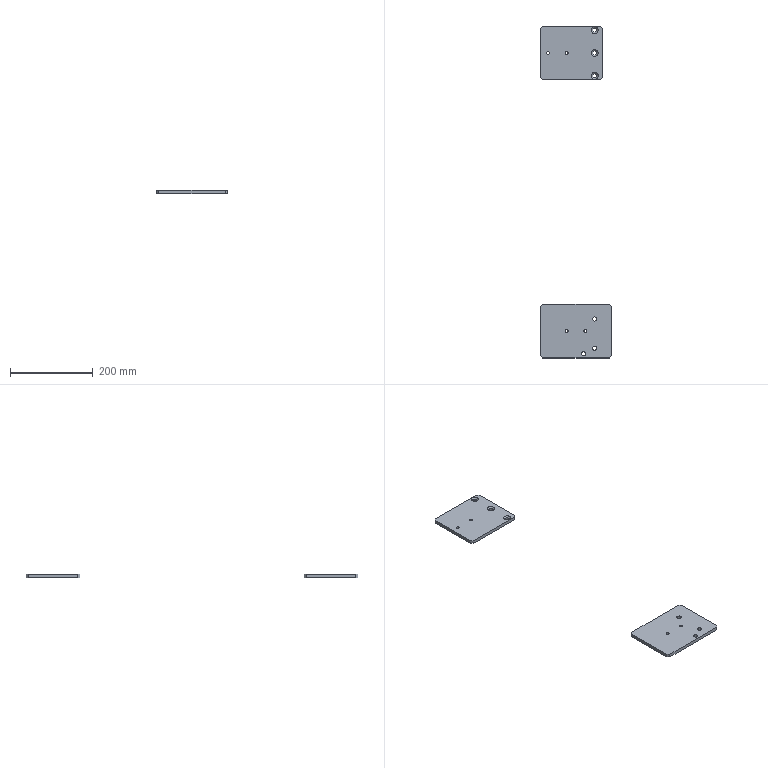Part | NX | features BREP 2 | 2 solids | 46 faces | box 170 x 800 x 8 mm | volume 326356 mm3 | cylinder 20 | plane 20 | cone 6 | commonest cylinder face diameters 10 x12 6.8 x8
STEP:
#1=CARTESIAN_POINT('',(23.429,-390.,0.));
#2=VERTEX_POINT('',#1);
#3=CARTESIAN_POINT('',(13.429,-390.,0.));
#4=VERTEX_POINT('',#3);
#5=CARTESIAN_POINT('',(18.429,-390.,0.));
#6=DIRECTION('',(0.,0.,-1.));
#7=DIRECTION('',(-1.,0.,0.));
#8=AXIS2_PLACEMENT_3D('',#5,#6,#7);
#9=CIRCLE('',#8,5.);
#10=EDGE_CURVE('',#2,#4,#9,.T.);
#11=ORIENTED_EDGE('',*,*,#10,.T.);
#12=CARTESIAN_POINT('',(13.429,-390.,8.));
#13=VERTEX_POINT('',#12);
#14=CARTESIAN_POINT('',(13.429,-390.,8.));
#15=DIRECTION('',(0.,0.,1.));
#16=VECTOR('',#15,1000.);
#17=LINE('',#14,#16);
#18=EDGE_CURVE('',#13,#4,#17,.F.);
#19=ORIENTED_EDGE('',*,*,#18,.F.);
#20=CARTESIAN_POINT('',(23.429,-390.,8.));
#21=VERTEX_POINT('',#20);
#22=CARTESIAN_POINT('',(18.429,-390.,8.));
#23=DIRECTION('',(0.,0.,1.));
#24=DIRECTION('',(1.,0.,0.));
#25=AXIS2_PLACEMENT_3D('',#22,#23,#24);
#26=CIRCLE('',#25,5.);
#27=EDGE_CURVE('',#13,#21,#26,.T.);
#28=ORIENTED_EDGE('',*,*,#27,.T.);
#29=CARTESIAN_POINT('',(23.429,-390.,8.));
#30=DIRECTION('',(0.,0.,1.));
#31=VECTOR('',#30,1000.);
#32=LINE('',#29,#31);
#33=EDGE_CURVE('',#21,#2,#32,.F.);
#34=ORIENTED_EDGE('',*,*,#33,.T.);
#35=EDGE_LOOP('',(#11,#19,#28,#34));
#36=FACE_BOUND('',#35,.T.);
#37=CARTESIAN_POINT('',(18.429,-390.,8.));
#38=DIRECTION('',(0.,0.,1.));
#39=DIRECTION('',(1.,0.,0.));
#40=AXIS2_PLACEMENT_3D('',#37,#38,#39);
#41=CYLINDRICAL_SURFACE('',#40,5.);
#42=ADVANCED_FACE('',(#36),#41,.F.);
#43=CARTESIAN_POINT('',(50.,-376.071,0.));
#44=VERTEX_POINT('',#43);
#45=CARTESIAN_POINT('',(40.,-376.071,0.));
#46=VERTEX_POINT('',#45);
#47=CARTESIAN_POINT('',(45.,-376.071,0.));
#48=DIRECTION('',(0.,0.,-1.));
#49=DIRECTION('',(-1.,0.,0.));
#50=AXIS2_PLACEMENT_3D('',#47,#48,#49);
#51=CIRCLE('',#50,5.);
#52=EDGE_CURVE('',#44,#46,#51,.T.);
#53=ORIENTED_EDGE('',*,*,#52,.T.);
#54=CARTESIAN_POINT('',(40.,-376.071,8.));
#55=VERTEX_POINT('',#54);
#56=CARTESIAN_POINT('',(40.,-376.071,8.));
#57=DIRECTION('',(0.,0.,1.));
#58=VECTOR('',#57,1000.);
#59=LINE('',#56,#58);
#60=EDGE_CURVE('',#55,#46,#59,.F.);
#61=ORIENTED_EDGE('',*,*,#60,.F.);
#62=CARTESIAN_POINT('',(50.,-376.071,8.));
#63=VERTEX_POINT('',#62);
#64=CARTESIAN_POINT('',(45.,-376.071,8.));
#65=DIRECTION('',(0.,0.,1.));
#66=DIRECTION('',(1.,0.,0.));
#67=AXIS2_PLACEMENT_3D('',#64,#65,#66);
#68=CIRCLE('',#67,5.);
#69=EDGE_CURVE('',#55,#63,#68,.T.);
#70=ORIENTED_EDGE('',*,*,#69,.T.);
#71=CARTESIAN_POINT('',(50.,-376.071,8.));
#72=DIRECTION('',(0.,0.,1.));
#73=VECTOR('',#72,1000.);
#74=LINE('',#71,#73);
#75=EDGE_CURVE('',#63,#44,#74,.F.);
#76=ORIENTED_EDGE('',*,*,#75,.T.);
#77=EDGE_LOOP('',(#53,#61,#70,#76));
#78=FACE_BOUND('',#77,.T.);
#79=CARTESIAN_POINT('',(45.,-376.071,8.));
#80=DIRECTION('',(0.,0.,1.));
#81=DIRECTION('',(1.,0.,0.));
#82=AXIS2_PLACEMENT_3D('',#79,#80,#81);
#83=CYLINDRICAL_SURFACE('',#82,5.);
#84=ADVANCED_FACE('',(#78),#83,.F.);
#85=CARTESIAN_POINT('',(50.,-306.071,0.));
#86=VERTEX_POINT('',#85);
#87=CARTESIAN_POINT('',(40.,-306.071,0.));
#88=VERTEX_POINT('',#87);
#89=CARTESIAN_POINT('',(45.,-306.071,0.));
#90=DIRECTION('',(0.,0.,-1.));
#91=DIRECTION('',(-1.,0.,0.));
#92=AXIS2_PLACEMENT_3D('',#89,#90,#91);
#93=CIRCLE('',#92,5.);
#94=EDGE_CURVE('',#86,#88,#93,.T.);
#95=ORIENTED_EDGE('',*,*,#94,.T.);
#96=CARTESIAN_POINT('',(40.,-306.071,8.));
#97=VERTEX_POINT('',#96);
#98=CARTESIAN_POINT('',(40.,-306.071,8.));
#99=DIRECTION('',(0.,0.,1.));
#100=VECTOR('',#99,1000.);
#101=LINE('',#98,#100);
#102=EDGE_CURVE('',#97,#88,#101,.F.);
#103=ORIENTED_EDGE('',*,*,#102,.F.);
#104=CARTESIAN_POINT('',(50.,-306.071,8.));
#105=VERTEX_POINT('',#104);
#106=CARTESIAN_POINT('',(45.,-306.071,8.));
#107=DIRECTION('',(0.,0.,1.));
#108=DIRECTION('',(1.,0.,0.));
#109=AXIS2_PLACEMENT_3D('',#106,#107,#108);
#110=CIRCLE('',#109,5.);
#111=EDGE_CURVE('',#97,#105,#110,.T.);
#112=ORIENTED_EDGE('',*,*,#111,.T.);
#113=CARTESIAN_POINT('',(50.,-306.071,8.));
#114=DIRECTION('',(0.,0.,1.));
#115=VECTOR('',#114,1000.);
#116=LINE('',#113,#115);
#117=EDGE_CURVE('',#105,#86,#116,.F.);
#118=ORIENTED_EDGE('',*,*,#117,.T.);
#119=EDGE_LOOP('',(#95,#103,#112,#118));
#120=FACE_BOUND('',#119,.T.);
#121=CARTESIAN_POINT('',(45.,-306.071,8.));
#122=DIRECTION('',(0.,0.,1.));
#123=DIRECTION('',(1.,0.,0.));
#124=AXIS2_PLACEMENT_3D('',#121,#122,#123);
#125=CYLINDRICAL_SURFACE('',#124,5.);
#126=ADVANCED_FACE('',(#120),#125,.F.);
#127=CARTESIAN_POINT('',(25.9,-335.,0.));
#128=VERTEX_POINT('',#127);
#129=CARTESIAN_POINT('',(19.1,-335.,0.));
#130=VERTEX_POINT('',#129);
#131=CARTESIAN_POINT('',(22.5,-335.,0.));
#132=DIRECTION('',(0.,0.,-1.));
#133=DIRECTION('',(-1.,0.,0.));
#134=AXIS2_PLACEMENT_3D('',#131,#132,#133);
#135=CIRCLE('',#134,3.4);
#136=EDGE_CURVE('',#128,#130,#135,.T.);
#137=ORIENTED_EDGE('',*,*,#136,.T.);
#138=CARTESIAN_POINT('',(19.1,-335.,8.));
#139=VERTEX_POINT('',#138);
#140=CARTESIAN_POINT('',(19.1,-335.,8.));
#141=DIRECTION('',(0.,0.,1.));
#142=VECTOR('',#141,1000.);
#143=LINE('',#140,#142);
#144=EDGE_CURVE('',#139,#130,#143,.F.);
#145=ORIENTED_EDGE('',*,*,#144,.F.);
#146=CARTESIAN_POINT('',(25.9,-335.,8.));
#147=VERTEX_POINT('',#146);
#148=CARTESIAN_POINT('',(22.5,-335.,8.));
#149=DIRECTION('',(0.,0.,1.));
#150=DIRECTION('',(1.,0.,0.));
#151=AXIS2_PLACEMENT_3D('',#148,#149,#150);
#152=CIRCLE('',#151,3.4);
#153=EDGE_CURVE('',#139,#147,#152,.T.);
#154=ORIENTED_EDGE('',*,*,#153,.T.);
#155=CARTESIAN_POINT('',(25.9,-335.,8.));
#156=DIRECTION('',(0.,0.,1.));
#157=VECTOR('',#156,1000.);
#158=LINE('',#155,#157);
#159=EDGE_CURVE('',#147,#128,#158,.F.);
#160=ORIENTED_EDGE('',*,*,#159,.T.);
#161=EDGE_LOOP('',(#137,#145,#154,#160));
#162=FACE_BOUND('',#161,.T.);
#163=CARTESIAN_POINT('',(22.5,-335.,8.));
#164=DIRECTION('',(0.,0.,1.));
#165=DIRECTION('',(1.,0.,0.));
#166=AXIS2_PLACEMENT_3D('',#163,#164,#165);
#167=CYLINDRICAL_SURFACE('',#166,3.4);
#168=ADVANCED_FACE('',(#162),#167,.F.);
#169=CARTESIAN_POINT('',(-19.1,-335.,0.));
#170=VERTEX_POINT('',#169);
#171=CARTESIAN_POINT('',(-25.9,-335.,0.));
#172=VERTEX_POINT('',#171);
#173=CARTESIAN_POINT('',(-22.5,-335.,0.));
#174=DIRECTION('',(0.,0.,-1.));
#175=DIRECTION('',(-1.,0.,0.));
#176=AXIS2_PLACEMENT_3D('',#173,#174,#175);
#177=CIRCLE('',#176,3.4);
#178=EDGE_CURVE('',#170,#172,#177,.T.);
#179=ORIENTED_EDGE('',*,*,#178,.T.);
#180=CARTESIAN_POINT('',(-25.9,-335.,8.));
#181=VERTEX_POINT('',#180);
#182=CARTESIAN_POINT('',(-25.9,-335.,8.));
#183=DIRECTION('',(0.,0.,1.));
#184=VECTOR('',#183,1000.);
#185=LINE('',#182,#184);
#186=EDGE_CURVE('',#181,#172,#185,.F.);
#187=ORIENTED_EDGE('',*,*,#186,.F.);
#188=CARTESIAN_POINT('',(-19.1,-335.,8.));
#189=VERTEX_POINT('',#188);
#190=CARTESIAN_POINT('',(-22.5,-335.,8.));
#191=DIRECTION('',(0.,0.,1.));
#192=DIRECTION('',(1.,0.,0.));
#193=AXIS2_PLACEMENT_3D('',#190,#191,#192);
#194=CIRCLE('',#193,3.4);
#195=EDGE_CURVE('',#181,#189,#194,.T.);
#196=ORIENTED_EDGE('',*,*,#195,.T.);
#197=CARTESIAN_POINT('',(-19.1,-335.,8.));
#198=DIRECTION('',(0.,0.,1.));
#199=VECTOR('',#198,1000.);
#200=LINE('',#197,#199);
#201=EDGE_CURVE('',#189,#170,#200,.F.);
#202=ORIENTED_EDGE('',*,*,#201,.T.);
#203=EDGE_LOOP('',(#179,#187,#196,#202));
#204=FACE_BOUND('',#203,.T.);
#205=CARTESIAN_POINT('',(-22.5,-335.,8.));
#206=DIRECTION('',(0.,0.,1.));
#207=DIRECTION('',(1.,0.,0.));
#208=AXIS2_PLACEMENT_3D('',#205,#206,#207);
#209=CYLINDRICAL_SURFACE('',#208,3.4);
#210=ADVANCED_FACE('',(#204),#209,.F.);
#211=CARTESIAN_POINT('',(85.,-395.,8.));
#212=VERTEX_POINT('',#211);
#213=CARTESIAN_POINT('',(85.,-275.,8.));
#214=VERTEX_POINT('',#213);
#215=CARTESIAN_POINT('',(85.,-400.,8.));
#216=DIRECTION('',(0.,1.,0.));
#217=VECTOR('',#216,1000.);
#218=LINE('',#215,#217);
#219=EDGE_CURVE('',#212,#214,#218,.T.);
#220=ORIENTED_EDGE('',*,*,#219,.F.);
#221=CARTESIAN_POINT('',(85.,-395.,0.));
#222=VERTEX_POINT('',#221);
#223=CARTESIAN_POINT('',(85.,-395.,8.));
#224=DIRECTION('',(0.,0.,-1.));
#225=VECTOR('',#224,1000.);
#226=LINE('',#223,#225);
#227=EDGE_CURVE('',#212,#222,#226,.T.);
#228=ORIENTED_EDGE('',*,*,#227,.T.);
#229=CARTESIAN_POINT('',(85.,-275.,0.));
#230=VERTEX_POINT('',#229);
#231=CARTESIAN_POINT('',(85.,-400.,0.));
#232=DIRECTION('',(0.,1.,0.));
#233=VECTOR('',#232,1000.);
#234=LINE('',#231,#233);
#235=EDGE_CURVE('',#222,#230,#234,.T.);
#236=ORIENTED_EDGE('',*,*,#235,.T.);
#237=CARTESIAN_POINT('',(85.,-275.,8.));
#238=DIRECTION('',(0.,0.,1.));
#239=VECTOR('',#238,1000.);
#240=LINE('',#237,#239);
#241=EDGE_CURVE('',#230,#214,#240,.T.);
#242=ORIENTED_EDGE('',*,*,#241,.T.);
#243=EDGE_LOOP('',(#220,#228,#236,#242));
#244=FACE_BOUND('',#243,.T.);
#245=CARTESIAN_POINT('',(85.,-400.,8.));
#246=DIRECTION('',(-1.,0.,0.));
#247=DIRECTION('',(0.,0.,1.));
#248=AXIS2_PLACEMENT_3D('',#245,#246,#247);
#249=PLANE('',#248);
#250=ADVANCED_FACE('',(#244),#249,.F.);
#251=CARTESIAN_POINT('',(-85.,-275.,0.));
#252=VERTEX_POINT('',#251);
#253=CARTESIAN_POINT('',(-85.,-395.,0.));
#254=VERTEX_POINT('',#253);
#255=CARTESIAN_POINT('',(-85.,-400.,0.));
#256=DIRECTION('',(0.,-1.,0.));
#257=VECTOR('',#256,1000.);
#258=LINE('',#255,#257);
#259=EDGE_CURVE('',#252,#254,#258,.T.);
#260=ORIENTED_EDGE('',*,*,#259,.T.);
#261=CARTESIAN_POINT('',(-85.,-395.,8.));
#262=VERTEX_POINT('',#261);
#263=CARTESIAN_POINT('',(-85.,-395.,8.));
#264=DIRECTION('',(0.,0.,1.));
#265=VECTOR('',#264,1000.);
#266=LINE('',#263,#265);
#267=EDGE_CURVE('',#254,#262,#266,.T.);
#268=ORIENTED_EDGE('',*,*,#267,.T.);
#269=CARTESIAN_POINT('',(-85.,-275.,8.));
#270=VERTEX_POINT('',#269);
#271=CARTESIAN_POINT('',(-85.,-400.,8.));
#272=DIRECTION('',(0.,-1.,0.));
#273=VECTOR('',#272,1000.);
#274=LINE('',#271,#273);
#275=EDGE_CURVE('',#270,#262,#274,.T.);
#276=ORIENTED_EDGE('',*,*,#275,.F.);
#277=CARTESIAN_POINT('',(-85.,-275.,8.));
#278=DIRECTION('',(0.,0.,-1.));
#279=VECTOR('',#278,1000.);
#280=LINE('',#277,#279);
#281=EDGE_CURVE('',#270,#252,#280,.T.);
#282=ORIENTED_EDGE('',*,*,#281,.T.);
#283=EDGE_LOOP('',(#260,#268,#276,#282));
#284=FACE_BOUND('',#283,.T.);
#285=CARTESIAN_POINT('',(-85.,-400.,8.));
#286=DIRECTION('',(1.,0.,0.));
#287=DIRECTION('',(0.,1.,0.));
#288=AXIS2_PLACEMENT_3D('',#285,#286,#287);
#289=PLANE('',#288);
#290=ADVANCED_FACE('',(#284),#289,.F.);
#291=CARTESIAN_POINT('',(-80.,-400.,8.));
#292=VERTEX_POINT('',#291);
#293=CARTESIAN_POINT('',(80.,-400.,8.));
#294=VERTEX_POINT('',#293);
#295=CARTESIAN_POINT('',(-85.,-400.,8.));
#296=DIRECTION('',(1.,0.,0.));
#297=VECTOR('',#296,1000.);
#298=LINE('',#295,#297);
#299=EDGE_CURVE('',#292,#294,#298,.T.);
#300=ORIENTED_EDGE('',*,*,#299,.T.);
#301=CARTESIAN_POINT('',(85.,-395.,8.));
#302=DIRECTION('',(0.7071,0.7071,0.));
#303=VECTOR('',#302,1000.);
#304=LINE('',#301,#303);
#305=EDGE_CURVE('',#294,#212,#304,.T.);
#306=ORIENTED_EDGE('',*,*,#305,.T.);
#307=ORIENTED_EDGE('',*,*,#219,.T.);
#308=CARTESIAN_POINT('',(80.,-270.,8.));
#309=VERTEX_POINT('',#308);
#310=CARTESIAN_POINT('',(85.,-275.,8.));
#311=DIRECTION('',(-0.7071,0.7071,0.));
#312=VECTOR('',#311,1000.);
#313=LINE('',#310,#312);
#314=EDGE_CURVE('',#214,#309,#313,.T.);
#315=ORIENTED_EDGE('',*,*,#314,.T.);
#316=CARTESIAN_POINT('',(-80.,-270.,8.));
#317=VERTEX_POINT('',#316);
#318=CARTESIAN_POINT('',(-85.,-270.,8.));
#319=DIRECTION('',(1.,0.,0.));
#320=VECTOR('',#319,1000.);
#321=LINE('',#318,#320);
#322=EDGE_CURVE('',#317,#309,#321,.T.);
#323=ORIENTED_EDGE('',*,*,#322,.F.);
#324=CARTESIAN_POINT('',(-80.,-270.,8.));
#325=DIRECTION('',(-0.7071,-0.7071,0.));
#326=VECTOR('',#325,1000.);
#327=LINE('',#324,#326);
#328=EDGE_CURVE('',#317,#270,#327,.T.);
#329=ORIENTED_EDGE('',*,*,#328,.T.);
#330=ORIENTED_EDGE('',*,*,#275,.T.);
#331=CARTESIAN_POINT('',(-80.,-400.,8.));
#332=DIRECTION('',(0.7071,-0.7071,0.));
#333=VECTOR('',#332,1000.);
#334=LINE('',#331,#333);
#335=EDGE_CURVE('',#262,#292,#334,.T.);
#336=ORIENTED_EDGE('',*,*,#335,.T.);
#337=EDGE_LOOP('',(#300,#306,#307,#315,#323,#329,#330,#336));
#338=FACE_BOUND('',#337,.T.);
#339=CARTESIAN_POINT('',(-22.5,-335.,8.));
#340=DIRECTION('',(0.,0.,1.));
#341=DIRECTION('',(1.,0.,0.));
#342=AXIS2_PLACEMENT_3D('',#339,#340,#341);
#343=CIRCLE('',#342,3.4);
#344=EDGE_CURVE('',#189,#181,#343,.T.);
#345=ORIENTED_EDGE('',*,*,#344,.F.);
#346=ORIENTED_EDGE('',*,*,#195,.F.);
#347=EDGE_LOOP('',(#345,#346));
#348=FACE_BOUND('',#347,.T.);
#349=CARTESIAN_POINT('',(22.5,-335.,8.));
#350=DIRECTION('',(0.,0.,1.));
#351=DIRECTION('',(1.,0.,0.));
#352=AXIS2_PLACEMENT_3D('',#349,#350,#351);
#353=CIRCLE('',#352,3.4);
#354=EDGE_CURVE('',#147,#139,#353,.T.);
#355=ORIENTED_EDGE('',*,*,#354,.F.);
#356=ORIENTED_EDGE('',*,*,#153,.F.);
#357=EDGE_LOOP('',(#355,#356));
#358=FACE_BOUND('',#357,.T.);
#359=CARTESIAN_POINT('',(45.,-306.071,8.));
#360=DIRECTION('',(0.,0.,1.));
#361=DIRECTION('',(1.,0.,0.));
#362=AXIS2_PLACEMENT_3D('',#359,#360,#361);
#363=CIRCLE('',#362,5.);
#364=EDGE_CURVE('',#105,#97,#363,.T.);
#365=ORIENTED_EDGE('',*,*,#364,.F.);
#366=ORIENTED_EDGE('',*,*,#111,.F.);
#367=EDGE_LOOP('',(#365,#366));
#368=FACE_BOUND('',#367,.T.);
#369=CARTESIAN_POINT('',(45.,-376.071,8.));
#370=DIRECTION('',(0.,0.,1.));
#371=DIRECTION('',(1.,0.,0.));
#372=AXIS2_PLACEMENT_3D('',#369,#370,#371);
#373=CIRCLE('',#372,5.);
#374=EDGE_CURVE('',#63,#55,#373,.T.);
#375=ORIENTED_EDGE('',*,*,#374,.F.);
#376=ORIENTED_EDGE('',*,*,#69,.F.);
#377=EDGE_LOOP('',(#375,#376));
#378=FACE_BOUND('',#377,.T.);
#379=CARTESIAN_POINT('',(18.429,-390.,8.));
#380=DIRECTION('',(0.,0.,1.));
#381=DIRECTION('',(1.,0.,0.));
#382=AXIS2_PLACEMENT_3D('',#379,#380,#381);
#383=CIRCLE('',#382,5.);
#384=EDGE_CURVE('',#21,#13,#383,.T.);
#385=ORIENTED_EDGE('',*,*,#384,.F.);
#386=ORIENTED_EDGE('',*,*,#27,.F.);
#387=EDGE_LOOP('',(#385,#386));
#388=FACE_BOUND('',#387,.T.);
#389=CARTESIAN_POINT('',(0.,0.,8.));
#390=DIRECTION('',(0.,0.,-1.));
#391=DIRECTION('',(0.,-1.,0.));
#392=AXIS2_PLACEMENT_3D('',#389,#390,#391);
#393=PLANE('',#392);
#394=ADVANCED_FACE('',(#338,#348,#358,#368,#378,#388),#393,.F.);
#395=ORIENTED_EDGE('',*,*,#235,.F.);
#396=CARTESIAN_POINT('',(80.,-400.,0.));
#397=VERTEX_POINT('',#396);
#398=CARTESIAN_POINT('',(240.,-240.,0.));
#399=DIRECTION('',(-0.7071,-0.7071,0.));
#400=VECTOR('',#399,1000.);
#401=LINE('',#398,#400);
#402=EDGE_CURVE('',#222,#397,#401,.T.);
#403=ORIENTED_EDGE('',*,*,#402,.T.);
#404=CARTESIAN_POINT('',(-80.,-400.,0.));
#405=VERTEX_POINT('',#404);
#406=CARTESIAN_POINT('',(-85.,-400.,0.));
#407=DIRECTION('',(1.,0.,0.));
#408=VECTOR('',#407,1000.);
#409=LINE('',#406,#408);
#410=EDGE_CURVE('',#405,#397,#409,.T.);
#411=ORIENTED_EDGE('',*,*,#410,.F.);
#412=CARTESIAN_POINT('',(-240.,-240.,0.));
#413=DIRECTION('',(-0.7071,0.7071,0.));
#414=VECTOR('',#413,1000.);
#415=LINE('',#412,#414);
#416=EDGE_CURVE('',#405,#254,#415,.T.);
#417=ORIENTED_EDGE('',*,*,#416,.T.);
#418=ORIENTED_EDGE('',*,*,#259,.F.);
#419=CARTESIAN_POINT('',(-80.,-270.,0.));
#420=VERTEX_POINT('',#419);
#421=CARTESIAN_POINT('',(95.,-95.,0.));
#422=DIRECTION('',(0.7071,0.7071,0.));
#423=VECTOR('',#422,1000.);
#424=LINE('',#421,#423);
#425=EDGE_CURVE('',#252,#420,#424,.T.);
#426=ORIENTED_EDGE('',*,*,#425,.T.);
#427=CARTESIAN_POINT('',(80.,-270.,0.));
#428=VERTEX_POINT('',#427);
#429=CARTESIAN_POINT('',(0.,-270.,0.));
#430=DIRECTION('',(-1.,0.,0.));
#431=VECTOR('',#430,1000.);
#432=LINE('',#429,#431);
#433=EDGE_CURVE('',#428,#420,#432,.T.);
#434=ORIENTED_EDGE('',*,*,#433,.F.);
#435=CARTESIAN_POINT('',(-95.,-95.,0.));
#436=DIRECTION('',(0.7071,-0.7071,0.));
#437=VECTOR('',#436,1000.);
#438=LINE('',#435,#437);
#439=EDGE_CURVE('',#428,#230,#438,.T.);
#440=ORIENTED_EDGE('',*,*,#439,.T.);
#441=EDGE_LOOP('',(#395,#403,#411,#417,#418,#426,#434,#440));
#442=FACE_BOUND('',#441,.T.);
#443=ORIENTED_EDGE('',*,*,#178,.F.);
#444=CARTESIAN_POINT('',(-22.5,-335.,0.));
#445=DIRECTION('',(0.,0.,-1.));
#446=DIRECTION('',(-1.,0.,0.));
#447=AXIS2_PLACEMENT_3D('',#444,#445,#446);
#448=CIRCLE('',#447,3.4);
#449=EDGE_CURVE('',#172,#170,#448,.T.);
#450=ORIENTED_EDGE('',*,*,#449,.F.);
#451=EDGE_LOOP('',(#443,#450));
#452=FACE_BOUND('',#451,.T.);
#453=ORIENTED_EDGE('',*,*,#136,.F.);
#454=CARTESIAN_POINT('',(22.5,-335.,0.));
#455=DIRECTION('',(0.,0.,-1.));
#456=DIRECTION('',(-1.,0.,0.));
#457=AXIS2_PLACEMENT_3D('',#454,#455,#456);
#458=CIRCLE('',#457,3.4);
#459=EDGE_CURVE('',#130,#128,#458,.T.);
#460=ORIENTED_EDGE('',*,*,#459,.F.);
#461=EDGE_LOOP('',(#453,#460));
#462=FACE_BOUND('',#461,.T.);
#463=ORIENTED_EDGE('',*,*,#94,.F.);
#464=CARTESIAN_POINT('',(45.,-306.071,0.));
#465=DIRECTION('',(0.,0.,-1.));
#466=DIRECTION('',(-1.,0.,0.));
#467=AXIS2_PLACEMENT_3D('',#464,#465,#466);
#468=CIRCLE('',#467,5.);
#469=EDGE_CURVE('',#88,#86,#468,.T.);
#470=ORIENTED_EDGE('',*,*,#469,.F.);
#471=EDGE_LOOP('',(#463,#470));
#472=FACE_BOUND('',#471,.T.);
#473=ORIENTED_EDGE('',*,*,#52,.F.);
#474=CARTESIAN_POINT('',(45.,-376.071,0.));
#475=DIRECTION('',(0.,0.,-1.));
#476=DIRECTION('',(-1.,0.,0.));
#477=AXIS2_PLACEMENT_3D('',#474,#475,#476);
#478=CIRCLE('',#477,5.);
#479=EDGE_CURVE('',#46,#44,#478,.T.);
#480=ORIENTED_EDGE('',*,*,#479,.F.);
#481=EDGE_LOOP('',(#473,#480));
#482=FACE_BOUND('',#481,.T.);
#483=ORIENTED_EDGE('',*,*,#10,.F.);
#484=CARTESIAN_POINT('',(18.429,-390.,0.));
#485=DIRECTION('',(0.,0.,-1.));
#486=DIRECTION('',(-1.,0.,0.));
#487=AXIS2_PLACEMENT_3D('',#484,#485,#486);
#488=CIRCLE('',#487,5.);
#489=EDGE_CURVE('',#4,#2,#488,.T.);
#490=ORIENTED_EDGE('',*,*,#489,.F.);
#491=EDGE_LOOP('',(#483,#490));
#492=FACE_BOUND('',#491,.T.);
#493=CARTESIAN_POINT('',(0.,0.,0.));
#494=DIRECTION('',(0.,0.,-1.));
#495=DIRECTION('',(0.,-1.,0.));
#496=AXIS2_PLACEMENT_3D('',#493,#494,#495);
#497=PLANE('',#496);
#498=ADVANCED_FACE('',(#442,#452,#462,#472,#482,#492),#497,.T.);
#499=ORIENTED_EDGE('',*,*,#410,.T.);
#500=CARTESIAN_POINT('',(80.,-400.,8.));
#501=DIRECTION('',(0.,0.,1.));
#502=VECTOR('',#501,1000.);
#503=LINE('',#500,#502);
#504=EDGE_CURVE('',#397,#294,#503,.T.);
#505=ORIENTED_EDGE('',*,*,#504,.T.);
#506=ORIENTED_EDGE('',*,*,#299,.F.);
#507=CARTESIAN_POINT('',(-80.,-400.,8.));
#508=DIRECTION('',(0.,0.,-1.));
#509=VECTOR('',#508,1000.);
#510=LINE('',#507,#509);
#511=EDGE_CURVE('',#292,#405,#510,.T.);
#512=ORIENTED_EDGE('',*,*,#511,.T.);
#513=EDGE_LOOP('',(#499,#505,#506,#512));
#514=FACE_BOUND('',#513,.T.);
#515=CARTESIAN_POINT('',(-85.,-400.,8.));
#516=DIRECTION('',(0.,1.,0.));
#517=DIRECTION('',(1.,0.,0.));
#518=AXIS2_PLACEMENT_3D('',#515,#516,#517);
#519=PLANE('',#518);
#520=ADVANCED_FACE('',(#514),#519,.F.);
#521=ORIENTED_EDGE('',*,*,#186,.T.);
#522=ORIENTED_EDGE('',*,*,#449,.T.);
#523=ORIENTED_EDGE('',*,*,#201,.F.);
#524=ORIENTED_EDGE('',*,*,#344,.T.);
#525=EDGE_LOOP('',(#521,#522,#523,#524));
#526=FACE_BOUND('',#525,.T.);
#527=CARTESIAN_POINT('',(-22.5,-335.,8.));
#528=DIRECTION('',(0.,0.,1.));
#529=DIRECTION('',(1.,0.,0.));
#530=AXIS2_PLACEMENT_3D('',#527,#528,#529);
#531=CYLINDRICAL_SURFACE('',#530,3.4);
#532=ADVANCED_FACE('',(#526),#531,.F.);
#533=ORIENTED_EDGE('',*,*,#144,.T.);
#534=ORIENTED_EDGE('',*,*,#459,.T.);
#535=ORIENTED_EDGE('',*,*,#159,.F.);
#536=ORIENTED_EDGE('',*,*,#354,.T.);
#537=EDGE_LOOP('',(#533,#534,#535,#536));
#538=FACE_BOUND('',#537,.T.);
#539=CARTESIAN_POINT('',(22.5,-335.,8.));
#540=DIRECTION('',(0.,0.,1.));
#541=DIRECTION('',(1.,0.,0.));
#542=AXIS2_PLACEMENT_3D('',#539,#540,#541);
#543=CYLINDRICAL_SURFACE('',#542,3.4);
#544=ADVANCED_FACE('',(#538),#543,.F.);
#545=ORIENTED_EDGE('',*,*,#102,.T.);
#546=ORIENTED_EDGE('',*,*,#469,.T.);
#547=ORIENTED_EDGE('',*,*,#117,.F.);
#548=ORIENTED_EDGE('',*,*,#364,.T.);
#549=EDGE_LOOP('',(#545,#546,#547,#548));
#550=FACE_BOUND('',#549,.T.);
#551=CARTESIAN_POINT('',(45.,-306.071,8.));
#552=DIRECTION('',(0.,0.,1.));
#553=DIRECTION('',(1.,0.,0.));
#554=AXIS2_PLACEMENT_3D('',#551,#552,#553);
#555=CYLINDRICAL_SURFACE('',#554,5.);
#556=ADVANCED_FACE('',(#550),#555,.F.);
#557=ORIENTED_EDGE('',*,*,#60,.T.);
#558=ORIENTED_EDGE('',*,*,#479,.T.);
#559=ORIENTED_EDGE('',*,*,#75,.F.);
#560=ORIENTED_EDGE('',*,*,#374,.T.);
#561=EDGE_LOOP('',(#557,#558,#559,#560));
#562=FACE_BOUND('',#561,.T.);
#563=CARTESIAN_POINT('',(45.,-376.071,8.));
#564=DIRECTION('',(0.,0.,1.));
#565=DIRECTION('',(1.,0.,0.));
#566=AXIS2_PLACEMENT_3D('',#563,#564,#565);
#567=CYLINDRICAL_SURFACE('',#566,5.);
#568=ADVANCED_FACE('',(#562),#567,.F.);
#569=ORIENTED_EDGE('',*,*,#18,.T.);
#570=ORIENTED_EDGE('',*,*,#489,.T.);
#571=ORIENTED_EDGE('',*,*,#33,.F.);
#572=ORIENTED_EDGE('',*,*,#384,.T.);
#573=EDGE_LOOP('',(#569,#570,#571,#572));
#574=FACE_BOUND('',#573,.T.);
#575=CARTESIAN_POINT('',(18.429,-390.,8.));
#576=DIRECTION('',(0.,0.,1.));
#577=DIRECTION('',(1.,0.,0.));
#578=AXIS2_PLACEMENT_3D('',#575,#576,#577);
#579=CYLINDRICAL_SURFACE('',#578,5.);
#580=ADVANCED_FACE('',(#574),#579,.F.);
#581=ORIENTED_EDGE('',*,*,#433,.T.);
#582=CARTESIAN_POINT('',(-80.,-270.,-2.));
#583=DIRECTION('',(0.,0.,1.));
#584=VECTOR('',#583,1000.);
#585=LINE('',#582,#584);
#586=EDGE_CURVE('',#420,#317,#585,.T.);
#587=ORIENTED_EDGE('',*,*,#586,.T.);
#588=ORIENTED_EDGE('',*,*,#322,.T.);
#589=CARTESIAN_POINT('',(80.,-270.,-2.));
#590=DIRECTION('',(0.,0.,-1.));
#591=VECTOR('',#590,1000.);
#592=LINE('',#589,#591);
#593=EDGE_CURVE('',#309,#428,#592,.T.);
#594=ORIENTED_EDGE('',*,*,#593,.T.);
#595=EDGE_LOOP('',(#581,#587,#588,#594));
#596=FACE_BOUND('',#595,.T.);
#597=CARTESIAN_POINT('',(-85.,-270.,-2.));
#598=DIRECTION('',(0.,-1.,0.));
#599=DIRECTION('',(0.,0.,-1.));
#600=AXIS2_PLACEMENT_3D('',#597,#598,#599);
#601=PLANE('',#600);
#602=ADVANCED_FACE('',(#596),#601,.F.);
#603=ORIENTED_EDGE('',*,*,#305,.F.);
#604=ORIENTED_EDGE('',*,*,#504,.F.);
#605=ORIENTED_EDGE('',*,*,#402,.F.);
#606=ORIENTED_EDGE('',*,*,#227,.F.);
#607=EDGE_LOOP('',(#603,#604,#605,#606));
#608=FACE_BOUND('',#607,.T.);
#609=CARTESIAN_POINT('',(85.,-395.,8.));
#610=DIRECTION('',(-0.7071,0.7071,0.));
#611=DIRECTION('',(0.,0.,1.));
#612=AXIS2_PLACEMENT_3D('',#609,#610,#611);
#613=PLANE('',#612);
#614=ADVANCED_FACE('',(#608),#613,.F.);
#615=ORIENTED_EDGE('',*,*,#335,.F.);
#616=ORIENTED_EDGE('',*,*,#267,.F.);
#617=ORIENTED_EDGE('',*,*,#416,.F.);
#618=ORIENTED_EDGE('',*,*,#511,.F.);
#619=EDGE_LOOP('',(#615,#616,#617,#618));
#620=FACE_BOUND('',#619,.T.);
#621=CARTESIAN_POINT('',(-80.,-400.,8.));
#622=DIRECTION('',(0.7071,0.7071,0.));
#623=DIRECTION('',(0.,0.,-1.));
#624=AXIS2_PLACEMENT_3D('',#621,#622,#623);
#625=PLANE('',#624);
#626=ADVANCED_FACE('',(#620),#625,.F.);
#627=ORIENTED_EDGE('',*,*,#425,.F.);
#628=ORIENTED_EDGE('',*,*,#281,.F.);
#629=ORIENTED_EDGE('',*,*,#328,.F.);
#630=ORIENTED_EDGE('',*,*,#586,.F.);
#631=EDGE_LOOP('',(#627,#628,#629,#630));
#632=FACE_BOUND('',#631,.T.);
#633=CARTESIAN_POINT('',(-80.,-270.,-2.));
#634=DIRECTION('',(0.7071,-0.7071,0.));
#635=DIRECTION('',(0.,0.,-1.));
#636=AXIS2_PLACEMENT_3D('',#633,#634,#635);
#637=PLANE('',#636);
#638=ADVANCED_FACE('',(#632),#637,.F.);
#639=ORIENTED_EDGE('',*,*,#439,.F.);
#640=ORIENTED_EDGE('',*,*,#593,.F.);
#641=ORIENTED_EDGE('',*,*,#314,.F.);
#642=ORIENTED_EDGE('',*,*,#241,.F.);
#643=EDGE_LOOP('',(#639,#640,#641,#642));
#644=FACE_BOUND('',#643,.T.);
#645=CARTESIAN_POINT('',(85.,-275.,8.));
#646=DIRECTION('',(-0.7071,-0.7071,0.));
#647=DIRECTION('',(-0.7071,0.7071,0.));
#648=AXIS2_PLACEMENT_3D('',#645,#646,#647);
#649=PLANE('',#648);
#650=ADVANCED_FACE('',(#644),#649,.F.);
#651=CLOSED_SHELL('',(#42,#84,#126,#168,#210,#250,#290,#394,#498,#520,#532,#544,#556,#568,#580,#602,#614,#626,#638,#650));
#652=MANIFOLD_SOLID_BREP('',#651);
#653=CARTESIAN_POINT('',(40.,390.,4.5));
#654=VERTEX_POINT('',#653);
#655=CARTESIAN_POINT('',(50.,390.,4.5));
#656=VERTEX_POINT('',#655);
#657=CARTESIAN_POINT('',(45.,390.,4.5));
#658=DIRECTION('',(0.,0.,1.));
#659=DIRECTION('',(-1.,0.,0.));
#660=AXIS2_PLACEMENT_3D('',#657,#658,#659);
#661=CIRCLE('',#660,5.);
#662=EDGE_CURVE('',#654,#656,#661,.T.);
#663=ORIENTED_EDGE('',*,*,#662,.F.);
#664=CARTESIAN_POINT('',(36.5,390.,8.));
#665=VERTEX_POINT('',#664);
#666=CARTESIAN_POINT('',(40.,390.,4.5));
#667=DIRECTION('',(-0.7071,0.,0.7071));
#668=VECTOR('',#667,1000.);
#669=LINE('',#666,#668);
#670=EDGE_CURVE('',#665,#654,#669,.F.);
#671=ORIENTED_EDGE('',*,*,#670,.F.);
#672=CARTESIAN_POINT('',(53.5,390.,8.));
#673=VERTEX_POINT('',#672);
#674=CARTESIAN_POINT('',(45.,390.,8.));
#675=DIRECTION('',(0.,0.,-1.));
#676=DIRECTION('',(-1.,0.,0.));
#677=AXIS2_PLACEMENT_3D('',#674,#675,#676);
#678=CIRCLE('',#677,8.5);
#679=EDGE_CURVE('',#673,#665,#678,.T.);
#680=ORIENTED_EDGE('',*,*,#679,.F.);
#681=CARTESIAN_POINT('',(50.,390.,4.5));
#682=DIRECTION('',(0.7071,0.,0.7071));
#683=VECTOR('',#682,1000.);
#684=LINE('',#681,#683);
#685=EDGE_CURVE('',#673,#656,#684,.F.);
#686=ORIENTED_EDGE('',*,*,#685,.T.);
#687=EDGE_LOOP('',(#663,#671,#680,#686));
#688=FACE_BOUND('',#687,.T.);
#689=CARTESIAN_POINT('',(45.,390.,4.5));
#690=DIRECTION('',(0.,0.,1.));
#691=DIRECTION('',(1.,0.,0.));
#692=AXIS2_PLACEMENT_3D('',#689,#690,#691);
#693=CONICAL_SURFACE('',#692,5.,0.7854);
#694=ADVANCED_FACE('',(#688),#693,.F.);
#695=CARTESIAN_POINT('',(40.,335.,4.5));
#696=VERTEX_POINT('',#695);
#697=CARTESIAN_POINT('',(50.,335.,4.5));
#698=VERTEX_POINT('',#697);
#699=CARTESIAN_POINT('',(45.,335.,4.5));
#700=DIRECTION('',(0.,0.,1.));
#701=DIRECTION('',(-1.,0.,0.));
#702=AXIS2_PLACEMENT_3D('',#699,#700,#701);
#703=CIRCLE('',#702,5.);
#704=EDGE_CURVE('',#696,#698,#703,.T.);
#705=ORIENTED_EDGE('',*,*,#704,.F.);
#706=CARTESIAN_POINT('',(36.5,335.,8.));
#707=VERTEX_POINT('',#706);
#708=CARTESIAN_POINT('',(40.,335.,4.5));
#709=DIRECTION('',(-0.7071,0.,0.7071));
#710=VECTOR('',#709,1000.);
#711=LINE('',#708,#710);
#712=EDGE_CURVE('',#707,#696,#711,.F.);
#713=ORIENTED_EDGE('',*,*,#712,.F.);
#714=CARTESIAN_POINT('',(53.5,335.,8.));
#715=VERTEX_POINT('',#714);
#716=CARTESIAN_POINT('',(45.,335.,8.));
#717=DIRECTION('',(0.,0.,-1.));
#718=DIRECTION('',(-1.,0.,0.));
#719=AXIS2_PLACEMENT_3D('',#716,#717,#718);
#720=CIRCLE('',#719,8.5);
#721=EDGE_CURVE('',#715,#707,#720,.T.);
#722=ORIENTED_EDGE('',*,*,#721,.F.);
#723=CARTESIAN_POINT('',(50.,335.,4.5));
#724=DIRECTION('',(0.7071,0.,0.7071));
#725=VECTOR('',#724,1000.);
#726=LINE('',#723,#725);
#727=EDGE_CURVE('',#715,#698,#726,.F.);
#728=ORIENTED_EDGE('',*,*,#727,.T.);
#729=EDGE_LOOP('',(#705,#713,#722,#728));
#730=FACE_BOUND('',#729,.T.);
#731=CARTESIAN_POINT('',(45.,335.,4.5));
#732=DIRECTION('',(0.,0.,1.));
#733=DIRECTION('',(1.,0.,0.));
#734=AXIS2_PLACEMENT_3D('',#731,#732,#733);
#735=CONICAL_SURFACE('',#734,5.,0.7854);
#736=ADVANCED_FACE('',(#730),#735,.F.);
#737=CARTESIAN_POINT('',(40.,280.,4.5));
#738=VERTEX_POINT('',#737);
#739=CARTESIAN_POINT('',(50.,280.,4.5));
#740=VERTEX_POINT('',#739);
#741=CARTESIAN_POINT('',(45.,280.,4.5));
#742=DIRECTION('',(0.,0.,1.));
#743=DIRECTION('',(-1.,0.,0.));
#744=AXIS2_PLACEMENT_3D('',#741,#742,#743);
#745=CIRCLE('',#744,5.);
#746=EDGE_CURVE('',#738,#740,#745,.T.);
#747=ORIENTED_EDGE('',*,*,#746,.F.);
#748=CARTESIAN_POINT('',(36.5,280.,8.));
#749=VERTEX_POINT('',#748);
#750=CARTESIAN_POINT('',(40.,280.,4.5));
#751=DIRECTION('',(-0.7071,0.,0.7071));
#752=VECTOR('',#751,1000.);
#753=LINE('',#750,#752);
#754=EDGE_CURVE('',#749,#738,#753,.F.);
#755=ORIENTED_EDGE('',*,*,#754,.F.);
#756=CARTESIAN_POINT('',(53.5,280.,8.));
#757=VERTEX_POINT('',#756);
#758=CARTESIAN_POINT('',(45.,280.,8.));
#759=DIRECTION('',(0.,0.,-1.));
#760=DIRECTION('',(-1.,0.,0.));
#761=AXIS2_PLACEMENT_3D('',#758,#759,#760);
#762=CIRCLE('',#761,8.5);
#763=EDGE_CURVE('',#757,#749,#762,.T.);
#764=ORIENTED_EDGE('',*,*,#763,.F.);
#765=CARTESIAN_POINT('',(50.,280.,4.5));
#766=DIRECTION('',(0.7071,0.,0.7071));
#767=VECTOR('',#766,1000.);
#768=LINE('',#765,#767);
#769=EDGE_CURVE('',#757,#740,#768,.F.);
#770=ORIENTED_EDGE('',*,*,#769,.T.);
#771=EDGE_LOOP('',(#747,#755,#764,#770));
#772=FACE_BOUND('',#771,.T.);
#773=CARTESIAN_POINT('',(45.,280.,4.5));
#774=DIRECTION('',(0.,0.,1.));
#775=DIRECTION('',(1.,0.,0.));
#776=AXIS2_PLACEMENT_3D('',#773,#774,#775);
#777=CONICAL_SURFACE('',#776,5.,0.7854);
#778=ADVANCED_FACE('',(#772),#777,.F.);
#779=CARTESIAN_POINT('',(50.,390.,0.));
#780=VERTEX_POINT('',#779);
#781=CARTESIAN_POINT('',(40.,390.,0.));
#782=VERTEX_POINT('',#781);
#783=CARTESIAN_POINT('',(45.,390.,0.));
#784=DIRECTION('',(0.,0.,-1.));
#785=DIRECTION('',(-1.,0.,0.));
#786=AXIS2_PLACEMENT_3D('',#783,#784,#785);
#787=CIRCLE('',#786,5.);
#788=EDGE_CURVE('',#780,#782,#787,.T.);
#789=ORIENTED_EDGE('',*,*,#788,.T.);
#790=CARTESIAN_POINT('',(40.,390.,8.));
#791=DIRECTION('',(0.,0.,1.));
#792=VECTOR('',#791,1000.);
#793=LINE('',#790,#792);
#794=EDGE_CURVE('',#654,#782,#793,.F.);
#795=ORIENTED_EDGE('',*,*,#794,.F.);
#796=ORIENTED_EDGE('',*,*,#662,.T.);
#797=CARTESIAN_POINT('',(50.,390.,8.));
#798=DIRECTION('',(0.,0.,1.));
#799=VECTOR('',#798,1000.);
#800=LINE('',#797,#799);
#801=EDGE_CURVE('',#656,#780,#800,.F.);
#802=ORIENTED_EDGE('',*,*,#801,.T.);
#803=EDGE_LOOP('',(#789,#795,#796,#802));
#804=FACE_BOUND('',#803,.T.);
#805=CARTESIAN_POINT('',(45.,390.,8.));
#806=DIRECTION('',(0.,0.,1.));
#807=DIRECTION('',(1.,0.,0.));
#808=AXIS2_PLACEMENT_3D('',#805,#806,#807);
#809=CYLINDRICAL_SURFACE('',#808,5.);
#810=ADVANCED_FACE('',(#804),#809,.F.);
#811=CARTESIAN_POINT('',(50.,335.,0.));
#812=VERTEX_POINT('',#811);
#813=CARTESIAN_POINT('',(40.,335.,0.));
#814=VERTEX_POINT('',#813);
#815=CARTESIAN_POINT('',(45.,335.,0.));
#816=DIRECTION('',(0.,0.,-1.));
#817=DIRECTION('',(-1.,0.,0.));
#818=AXIS2_PLACEMENT_3D('',#815,#816,#817);
#819=CIRCLE('',#818,5.);
#820=EDGE_CURVE('',#812,#814,#819,.T.);
#821=ORIENTED_EDGE('',*,*,#820,.T.);
#822=CARTESIAN_POINT('',(40.,335.,8.));
#823=DIRECTION('',(0.,0.,1.));
#824=VECTOR('',#823,1000.);
#825=LINE('',#822,#824);
#826=EDGE_CURVE('',#696,#814,#825,.F.);
#827=ORIENTED_EDGE('',*,*,#826,.F.);
#828=ORIENTED_EDGE('',*,*,#704,.T.);
#829=CARTESIAN_POINT('',(50.,335.,8.));
#830=DIRECTION('',(0.,0.,1.));
#831=VECTOR('',#830,1000.);
#832=LINE('',#829,#831);
#833=EDGE_CURVE('',#698,#812,#832,.F.);
#834=ORIENTED_EDGE('',*,*,#833,.T.);
#835=EDGE_LOOP('',(#821,#827,#828,#834));
#836=FACE_BOUND('',#835,.T.);
#837=CARTESIAN_POINT('',(45.,335.,8.));
#838=DIRECTION('',(0.,0.,1.));
#839=DIRECTION('',(1.,0.,0.));
#840=AXIS2_PLACEMENT_3D('',#837,#838,#839);
#841=CYLINDRICAL_SURFACE('',#840,5.);
#842=ADVANCED_FACE('',(#836),#841,.F.);
#843=CARTESIAN_POINT('',(50.,280.,0.));
#844=VERTEX_POINT('',#843);
#845=CARTESIAN_POINT('',(40.,280.,0.));
#846=VERTEX_POINT('',#845);
#847=CARTESIAN_POINT('',(45.,280.,0.));
#848=DIRECTION('',(0.,0.,-1.));
#849=DIRECTION('',(-1.,0.,0.));
#850=AXIS2_PLACEMENT_3D('',#847,#848,#849);
#851=CIRCLE('',#850,5.);
#852=EDGE_CURVE('',#844,#846,#851,.T.);
#853=ORIENTED_EDGE('',*,*,#852,.T.);
#854=CARTESIAN_POINT('',(40.,280.,8.));
#855=DIRECTION('',(0.,0.,1.));
#856=VECTOR('',#855,1000.);
#857=LINE('',#854,#856);
#858=EDGE_CURVE('',#738,#846,#857,.F.);
#859=ORIENTED_EDGE('',*,*,#858,.F.);
#860=ORIENTED_EDGE('',*,*,#746,.T.);
#861=CARTESIAN_POINT('',(50.,280.,8.));
#862=DIRECTION('',(0.,0.,1.));
#863=VECTOR('',#862,1000.);
#864=LINE('',#861,#863);
#865=EDGE_CURVE('',#740,#844,#864,.F.);
#866=ORIENTED_EDGE('',*,*,#865,.T.);
#867=EDGE_LOOP('',(#853,#859,#860,#866));
#868=FACE_BOUND('',#867,.T.);
#869=CARTESIAN_POINT('',(45.,280.,8.));
#870=DIRECTION('',(0.,0.,1.));
#871=DIRECTION('',(1.,0.,0.));
#872=AXIS2_PLACEMENT_3D('',#869,#870,#871);
#873=CYLINDRICAL_SURFACE('',#872,5.);
#874=ADVANCED_FACE('',(#868),#873,.F.);
#875=CARTESIAN_POINT('',(-64.1,335.,0.));
#876=VERTEX_POINT('',#875);
#877=CARTESIAN_POINT('',(-70.9,335.,0.));
#878=VERTEX_POINT('',#877);
#879=CARTESIAN_POINT('',(-67.5,335.,0.));
#880=DIRECTION('',(0.,0.,-1.));
#881=DIRECTION('',(-1.,0.,0.));
#882=AXIS2_PLACEMENT_3D('',#879,#880,#881);
#883=CIRCLE('',#882,3.4);
#884=EDGE_CURVE('',#876,#878,#883,.T.);
#885=ORIENTED_EDGE('',*,*,#884,.T.);
#886=CARTESIAN_POINT('',(-70.9,335.,8.));
#887=VERTEX_POINT('',#886);
#888=CARTESIAN_POINT('',(-70.9,335.,8.));
#889=DIRECTION('',(0.,0.,1.));
#890=VECTOR('',#889,1000.);
#891=LINE('',#888,#890);
#892=EDGE_CURVE('',#887,#878,#891,.F.);
#893=ORIENTED_EDGE('',*,*,#892,.F.);
#894=CARTESIAN_POINT('',(-64.1,335.,8.));
#895=VERTEX_POINT('',#894);
#896=CARTESIAN_POINT('',(-67.5,335.,8.));
#897=DIRECTION('',(0.,0.,1.));
#898=DIRECTION('',(1.,0.,0.));
#899=AXIS2_PLACEMENT_3D('',#896,#897,#898);
#900=CIRCLE('',#899,3.4);
#901=EDGE_CURVE('',#887,#895,#900,.T.);
#902=ORIENTED_EDGE('',*,*,#901,.T.);
#903=CARTESIAN_POINT('',(-64.1,335.,8.));
#904=DIRECTION('',(0.,0.,1.));
#905=VECTOR('',#904,1000.);
#906=LINE('',#903,#905);
#907=EDGE_CURVE('',#895,#876,#906,.F.);
#908=ORIENTED_EDGE('',*,*,#907,.T.);
#909=EDGE_LOOP('',(#885,#893,#902,#908));
#910=FACE_BOUND('',#909,.T.);
#911=CARTESIAN_POINT('',(-67.5,335.,8.));
#912=DIRECTION('',(0.,0.,1.));
#913=DIRECTION('',(1.,0.,0.));
#914=AXIS2_PLACEMENT_3D('',#911,#912,#913);
#915=CYLINDRICAL_SURFACE('',#914,3.4);
#916=ADVANCED_FACE('',(#910),#915,.F.);
#917=CARTESIAN_POINT('',(-19.1,335.,0.));
#918=VERTEX_POINT('',#917);
#919=CARTESIAN_POINT('',(-25.9,335.,0.));
#920=VERTEX_POINT('',#919);
#921=CARTESIAN_POINT('',(-22.5,335.,0.));
#922=DIRECTION('',(0.,0.,-1.));
#923=DIRECTION('',(-1.,0.,0.));
#924=AXIS2_PLACEMENT_3D('',#921,#922,#923);
#925=CIRCLE('',#924,3.4);
#926=EDGE_CURVE('',#918,#920,#925,.T.);
#927=ORIENTED_EDGE('',*,*,#926,.T.);
#928=CARTESIAN_POINT('',(-25.9,335.,8.));
#929=VERTEX_POINT('',#928);
#930=CARTESIAN_POINT('',(-25.9,335.,8.));
#931=DIRECTION('',(0.,0.,1.));
#932=VECTOR('',#931,1000.);
#933=LINE('',#930,#932);
#934=EDGE_CURVE('',#929,#920,#933,.F.);
#935=ORIENTED_EDGE('',*,*,#934,.F.);
#936=CARTESIAN_POINT('',(-19.1,335.,8.));
#937=VERTEX_POINT('',#936);
#938=CARTESIAN_POINT('',(-22.5,335.,8.));
#939=DIRECTION('',(0.,0.,1.));
#940=DIRECTION('',(1.,0.,0.));
#941=AXIS2_PLACEMENT_3D('',#938,#939,#940);
#942=CIRCLE('',#941,3.4);
#943=EDGE_CURVE('',#929,#937,#942,.T.);
#944=ORIENTED_EDGE('',*,*,#943,.T.);
#945=CARTESIAN_POINT('',(-19.1,335.,8.));
#946=DIRECTION('',(0.,0.,1.));
#947=VECTOR('',#946,1000.);
#948=LINE('',#945,#947);
#949=EDGE_CURVE('',#937,#918,#948,.F.);
#950=ORIENTED_EDGE('',*,*,#949,.T.);
#951=EDGE_LOOP('',(#927,#935,#944,#950));
#952=FACE_BOUND('',#951,.T.);
#953=CARTESIAN_POINT('',(-22.5,335.,8.));
#954=DIRECTION('',(0.,0.,1.));
#955=DIRECTION('',(1.,0.,0.));
#956=AXIS2_PLACEMENT_3D('',#953,#954,#955);
#957=CYLINDRICAL_SURFACE('',#956,3.4);
#958=ADVANCED_FACE('',(#952),#957,.F.);
#959=CARTESIAN_POINT('',(60.,400.,8.));
#960=VERTEX_POINT('',#959);
#961=CARTESIAN_POINT('',(-80.,400.,8.));
#962=VERTEX_POINT('',#961);
#963=CARTESIAN_POINT('',(-85.,400.,8.));
#964=DIRECTION('',(-1.,0.,0.));
#965=VECTOR('',#964,1000.);
#966=LINE('',#963,#965);
#967=EDGE_CURVE('',#960,#962,#966,.T.);
#968=ORIENTED_EDGE('',*,*,#967,.F.);
#969=CARTESIAN_POINT('',(60.,400.,0.));
#970=VERTEX_POINT('',#969);
#971=CARTESIAN_POINT('',(60.,400.,0.));
#972=DIRECTION('',(0.,0.,-1.));
#973=VECTOR('',#972,1000.);
#974=LINE('',#971,#973);
#975=EDGE_CURVE('',#960,#970,#974,.T.);
#976=ORIENTED_EDGE('',*,*,#975,.T.);
#977=CARTESIAN_POINT('',(-80.,400.,0.));
#978=VERTEX_POINT('',#977);
#979=CARTESIAN_POINT('',(-85.,400.,0.));
#980=DIRECTION('',(-1.,0.,0.));
#981=VECTOR('',#980,1000.);
#982=LINE('',#979,#981);
#983=EDGE_CURVE('',#970,#978,#982,.T.);
#984=ORIENTED_EDGE('',*,*,#983,.T.);
#985=CARTESIAN_POINT('',(-80.,400.,8.));
#986=DIRECTION('',(0.,0.,1.));
#987=VECTOR('',#986,1000.);
#988=LINE('',#985,#987);
#989=EDGE_CURVE('',#978,#962,#988,.T.);
#990=ORIENTED_EDGE('',*,*,#989,.T.);
#991=EDGE_LOOP('',(#968,#976,#984,#990));
#992=FACE_BOUND('',#991,.T.);
#993=CARTESIAN_POINT('',(-85.,400.,8.));
#994=DIRECTION('',(0.,-1.,0.));
#995=DIRECTION('',(0.,0.,-1.));
#996=AXIS2_PLACEMENT_3D('',#993,#994,#995);
#997=PLANE('',#996);
#998=ADVANCED_FACE('',(#992),#997,.F.);
#999=CARTESIAN_POINT('',(60.,270.,8.));
#1000=VERTEX_POINT('',#999);
#1001=CARTESIAN_POINT('',(-80.,270.,8.));
#1002=VERTEX_POINT('',#1001);
#1003=CARTESIAN_POINT('',(-85.,270.,8.));
#1004=DIRECTION('',(-1.,0.,0.));
#1005=VECTOR('',#1004,1000.);
#1006=LINE('',#1003,#1005);
#1007=EDGE_CURVE('',#1000,#1002,#1006,.T.);
#1008=ORIENTED_EDGE('',*,*,#1007,.F.);
#1009=CARTESIAN_POINT('',(65.,275.,8.));
#1010=VERTEX_POINT('',#1009);
#1011=CARTESIAN_POINT('',(65.,275.,8.));
#1012=DIRECTION('',(0.7071,0.7071,0.));
#1013=VECTOR('',#1012,1000.);
#1014=LINE('',#1011,#1013);
#1015=EDGE_CURVE('',#1000,#1010,#1014,.T.);
#1016=ORIENTED_EDGE('',*,*,#1015,.T.);
#1017=CARTESIAN_POINT('',(65.,395.,8.));
#1018=VERTEX_POINT('',#1017);
#1019=CARTESIAN_POINT('',(65.,0.,8.));
#1020=DIRECTION('',(0.,-1.,0.));
#1021=VECTOR('',#1020,1000.);
#1022=LINE('',#1019,#1021);
#1023=EDGE_CURVE('',#1018,#1010,#1022,.T.);
#1024=ORIENTED_EDGE('',*,*,#1023,.F.);
#1025=CARTESIAN_POINT('',(65.,395.,8.));
#1026=DIRECTION('',(-0.7071,0.7071,0.));
#1027=VECTOR('',#1026,1000.);
#1028=LINE('',#1025,#1027);
#1029=EDGE_CURVE('',#1018,#960,#1028,.T.);
#1030=ORIENTED_EDGE('',*,*,#1029,.T.);
#1031=ORIENTED_EDGE('',*,*,#967,.T.);
#1032=CARTESIAN_POINT('',(-85.,395.,8.));
#1033=VERTEX_POINT('',#1032);
#1034=CARTESIAN_POINT('',(-85.,395.,8.));
#1035=DIRECTION('',(-0.7071,-0.7071,0.));
#1036=VECTOR('',#1035,1000.);
#1037=LINE('',#1034,#1036);
#1038=EDGE_CURVE('',#962,#1033,#1037,.T.);
#1039=ORIENTED_EDGE('',*,*,#1038,.T.);
#1040=CARTESIAN_POINT('',(-85.,275.,8.));
#1041=VERTEX_POINT('',#1040);
#1042=CARTESIAN_POINT('',(-85.,-400.,8.));
#1043=DIRECTION('',(0.,-1.,0.));
#1044=VECTOR('',#1043,1000.);
#1045=LINE('',#1042,#1044);
#1046=EDGE_CURVE('',#1033,#1041,#1045,.T.);
#1047=ORIENTED_EDGE('',*,*,#1046,.T.);
#1048=CARTESIAN_POINT('',(-85.,275.,8.));
#1049=DIRECTION('',(0.7071,-0.7071,0.));
#1050=VECTOR('',#1049,1000.);
#1051=LINE('',#1048,#1050);
#1052=EDGE_CURVE('',#1041,#1002,#1051,.T.);
#1053=ORIENTED_EDGE('',*,*,#1052,.T.);
#1054=EDGE_LOOP('',(#1008,#1016,#1024,#1030,#1031,#1039,#1047,#1053));
#1055=FACE_BOUND('',#1054,.T.);
#1056=CARTESIAN_POINT('',(-22.5,335.,8.));
#1057=DIRECTION('',(0.,0.,1.));
#1058=DIRECTION('',(1.,0.,0.));
#1059=AXIS2_PLACEMENT_3D('',#1056,#1057,#1058);
#1060=CIRCLE('',#1059,3.4);
#1061=EDGE_CURVE('',#937,#929,#1060,.T.);
#1062=ORIENTED_EDGE('',*,*,#1061,.F.);
#1063=ORIENTED_EDGE('',*,*,#943,.F.);
#1064=EDGE_LOOP('',(#1062,#1063));
#1065=FACE_BOUND('',#1064,.T.);
#1066=CARTESIAN_POINT('',(-67.5,335.,8.));
#1067=DIRECTION('',(0.,0.,1.));
#1068=DIRECTION('',(1.,0.,0.));
#1069=AXIS2_PLACEMENT_3D('',#1066,#1067,#1068);
#1070=CIRCLE('',#1069,3.4);
#1071=EDGE_CURVE('',#895,#887,#1070,.T.);
#1072=ORIENTED_EDGE('',*,*,#1071,.F.);
#1073=ORIENTED_EDGE('',*,*,#901,.F.);
#1074=EDGE_LOOP('',(#1072,#1073));
#1075=FACE_BOUND('',#1074,.T.);
#1076=ORIENTED_EDGE('',*,*,#679,.T.);
#1077=CARTESIAN_POINT('',(45.,390.,8.));
#1078=DIRECTION('',(0.,0.,-1.));
#1079=DIRECTION('',(-1.,0.,0.));
#1080=AXIS2_PLACEMENT_3D('',#1077,#1078,#1079);
#1081=CIRCLE('',#1080,8.5);
#1082=EDGE_CURVE('',#665,#673,#1081,.T.);
#1083=ORIENTED_EDGE('',*,*,#1082,.T.);
#1084=EDGE_LOOP('',(#1076,#1083));
#1085=FACE_BOUND('',#1084,.T.);
#1086=ORIENTED_EDGE('',*,*,#721,.T.);
#1087=CARTESIAN_POINT('',(45.,335.,8.));
#1088=DIRECTION('',(0.,0.,-1.));
#1089=DIRECTION('',(-1.,0.,0.));
#1090=AXIS2_PLACEMENT_3D('',#1087,#1088,#1089);
#1091=CIRCLE('',#1090,8.5);
#1092=EDGE_CURVE('',#707,#715,#1091,.T.);
#1093=ORIENTED_EDGE('',*,*,#1092,.T.);
#1094=EDGE_LOOP('',(#1086,#1093));
#1095=FACE_BOUND('',#1094,.T.);
#1096=ORIENTED_EDGE('',*,*,#763,.T.);
#1097=CARTESIAN_POINT('',(45.,280.,8.));
#1098=DIRECTION('',(0.,0.,-1.));
#1099=DIRECTION('',(-1.,0.,0.));
#1100=AXIS2_PLACEMENT_3D('',#1097,#1098,#1099);
#1101=CIRCLE('',#1100,8.5);
#1102=EDGE_CURVE('',#749,#757,#1101,.T.);
#1103=ORIENTED_EDGE('',*,*,#1102,.T.);
#1104=EDGE_LOOP('',(#1096,#1103));
#1105=FACE_BOUND('',#1104,.T.);
#1106=CARTESIAN_POINT('',(0.,0.,8.));
#1107=DIRECTION('',(0.,0.,-1.));
#1108=DIRECTION('',(0.,-1.,0.));
#1109=AXIS2_PLACEMENT_3D('',#1106,#1107,#1108);
#1110=PLANE('',#1109);
#1111=ADVANCED_FACE('',(#1055,#1065,#1075,#1085,#1095,#1105),#1110,.F.);
#1112=CARTESIAN_POINT('',(65.,395.,0.));
#1113=VERTEX_POINT('',#1112);
#1114=CARTESIAN_POINT('',(65.,275.,0.));
#1115=VERTEX_POINT('',#1114);
#1116=CARTESIAN_POINT('',(65.,0.,0.));
#1117=DIRECTION('',(0.,-1.,0.));
#1118=VECTOR('',#1117,1000.);
#1119=LINE('',#1116,#1118);
#1120=EDGE_CURVE('',#1113,#1115,#1119,.T.);
#1121=ORIENTED_EDGE('',*,*,#1120,.T.);
#1122=CARTESIAN_POINT('',(60.,270.,0.));
#1123=VERTEX_POINT('',#1122);
#1124=CARTESIAN_POINT('',(-105.,105.,0.));
#1125=DIRECTION('',(-0.7071,-0.7071,0.));
#1126=VECTOR('',#1125,1000.);
#1127=LINE('',#1124,#1126);
#1128=EDGE_CURVE('',#1115,#1123,#1127,.T.);
#1129=ORIENTED_EDGE('',*,*,#1128,.T.);
#1130=CARTESIAN_POINT('',(-80.,270.,0.));
#1131=VERTEX_POINT('',#1130);
#1132=CARTESIAN_POINT('',(0.,270.,0.));
#1133=DIRECTION('',(1.,0.,0.));
#1134=VECTOR('',#1133,1000.);
#1135=LINE('',#1132,#1134);
#1136=EDGE_CURVE('',#1131,#1123,#1135,.T.);
#1137=ORIENTED_EDGE('',*,*,#1136,.F.);
#1138=CARTESIAN_POINT('',(-85.,275.,0.));
#1139=VERTEX_POINT('',#1138);
#1140=CARTESIAN_POINT('',(95.,95.,0.));
#1141=DIRECTION('',(-0.7071,0.7071,0.));
#1142=VECTOR('',#1141,1000.);
#1143=LINE('',#1140,#1142);
#1144=EDGE_CURVE('',#1131,#1139,#1143,.T.);
#1145=ORIENTED_EDGE('',*,*,#1144,.T.);
#1146=CARTESIAN_POINT('',(-85.,395.,0.));
#1147=VERTEX_POINT('',#1146);
#1148=CARTESIAN_POINT('',(-85.,-400.,0.));
#1149=DIRECTION('',(0.,-1.,0.));
#1150=VECTOR('',#1149,1000.);
#1151=LINE('',#1148,#1150);
#1152=EDGE_CURVE('',#1147,#1139,#1151,.T.);
#1153=ORIENTED_EDGE('',*,*,#1152,.F.);
#1154=CARTESIAN_POINT('',(-240.,240.,0.));
#1155=DIRECTION('',(0.7071,0.7071,0.));
#1156=VECTOR('',#1155,1000.);
#1157=LINE('',#1154,#1156);
#1158=EDGE_CURVE('',#1147,#978,#1157,.T.);
#1159=ORIENTED_EDGE('',*,*,#1158,.T.);
#1160=ORIENTED_EDGE('',*,*,#983,.F.);
#1161=CARTESIAN_POINT('',(230.,230.,0.));
#1162=DIRECTION('',(0.7071,-0.7071,0.));
#1163=VECTOR('',#1162,1000.);
#1164=LINE('',#1161,#1163);
#1165=EDGE_CURVE('',#970,#1113,#1164,.T.);
#1166=ORIENTED_EDGE('',*,*,#1165,.T.);
#1167=EDGE_LOOP('',(#1121,#1129,#1137,#1145,#1153,#1159,#1160,#1166));
#1168=FACE_BOUND('',#1167,.T.);
#1169=ORIENTED_EDGE('',*,*,#788,.F.);
#1170=CARTESIAN_POINT('',(45.,390.,0.));
#1171=DIRECTION('',(0.,0.,-1.));
#1172=DIRECTION('',(-1.,0.,0.));
#1173=AXIS2_PLACEMENT_3D('',#1170,#1171,#1172);
#1174=CIRCLE('',#1173,5.);
#1175=EDGE_CURVE('',#782,#780,#1174,.T.);
#1176=ORIENTED_EDGE('',*,*,#1175,.F.);
#1177=EDGE_LOOP('',(#1169,#1176));
#1178=FACE_BOUND('',#1177,.T.);
#1179=ORIENTED_EDGE('',*,*,#820,.F.);
#1180=CARTESIAN_POINT('',(45.,335.,0.));
#1181=DIRECTION('',(0.,0.,-1.));
#1182=DIRECTION('',(-1.,0.,0.));
#1183=AXIS2_PLACEMENT_3D('',#1180,#1181,#1182);
#1184=CIRCLE('',#1183,5.);
#1185=EDGE_CURVE('',#814,#812,#1184,.T.);
#1186=ORIENTED_EDGE('',*,*,#1185,.F.);
#1187=EDGE_LOOP('',(#1179,#1186));
#1188=FACE_BOUND('',#1187,.T.);
#1189=ORIENTED_EDGE('',*,*,#852,.F.);
#1190=CARTESIAN_POINT('',(45.,280.,0.));
#1191=DIRECTION('',(0.,0.,-1.));
#1192=DIRECTION('',(-1.,0.,0.));
#1193=AXIS2_PLACEMENT_3D('',#1190,#1191,#1192);
#1194=CIRCLE('',#1193,5.);
#1195=EDGE_CURVE('',#846,#844,#1194,.T.);
#1196=ORIENTED_EDGE('',*,*,#1195,.F.);
#1197=EDGE_LOOP('',(#1189,#1196));
#1198=FACE_BOUND('',#1197,.T.);
#1199=ORIENTED_EDGE('',*,*,#884,.F.);
#1200=CARTESIAN_POINT('',(-67.5,335.,0.));
#1201=DIRECTION('',(0.,0.,-1.));
#1202=DIRECTION('',(-1.,0.,0.));
#1203=AXIS2_PLACEMENT_3D('',#1200,#1201,#1202);
#1204=CIRCLE('',#1203,3.4);
#1205=EDGE_CURVE('',#878,#876,#1204,.T.);
#1206=ORIENTED_EDGE('',*,*,#1205,.F.);
#1207=EDGE_LOOP('',(#1199,#1206));
#1208=FACE_BOUND('',#1207,.T.);
#1209=ORIENTED_EDGE('',*,*,#926,.F.);
#1210=CARTESIAN_POINT('',(-22.5,335.,0.));
#1211=DIRECTION('',(0.,0.,-1.));
#1212=DIRECTION('',(-1.,0.,0.));
#1213=AXIS2_PLACEMENT_3D('',#1210,#1211,#1212);
#1214=CIRCLE('',#1213,3.4);
#1215=EDGE_CURVE('',#920,#918,#1214,.T.);
#1216=ORIENTED_EDGE('',*,*,#1215,.F.);
#1217=EDGE_LOOP('',(#1209,#1216));
#1218=FACE_BOUND('',#1217,.T.);
#1219=CARTESIAN_POINT('',(0.,0.,0.));
#1220=DIRECTION('',(0.,0.,-1.));
#1221=DIRECTION('',(0.,-1.,0.));
#1222=AXIS2_PLACEMENT_3D('',#1219,#1220,#1221);
#1223=PLANE('',#1222);
#1224=ADVANCED_FACE('',(#1168,#1178,#1188,#1198,#1208,#1218),#1223,.T.);
#1225=ORIENTED_EDGE('',*,*,#1136,.T.);
#1226=CARTESIAN_POINT('',(60.,270.,8.));
#1227=DIRECTION('',(0.,0.,1.));
#1228=VECTOR('',#1227,1000.);
#1229=LINE('',#1226,#1228);
#1230=EDGE_CURVE('',#1123,#1000,#1229,.T.);
#1231=ORIENTED_EDGE('',*,*,#1230,.T.);
#1232=ORIENTED_EDGE('',*,*,#1007,.T.);
#1233=CARTESIAN_POINT('',(-80.,270.,-2.));
#1234=DIRECTION('',(0.,0.,-1.));
#1235=VECTOR('',#1234,1000.);
#1236=LINE('',#1233,#1235);
#1237=EDGE_CURVE('',#1002,#1131,#1236,.T.);
#1238=ORIENTED_EDGE('',*,*,#1237,.T.);
#1239=EDGE_LOOP('',(#1225,#1231,#1232,#1238));
#1240=FACE_BOUND('',#1239,.T.);
#1241=CARTESIAN_POINT('',(-85.,270.,-2.));
#1242=DIRECTION('',(0.,1.,0.));
#1243=DIRECTION('',(1.,0.,0.));
#1244=AXIS2_PLACEMENT_3D('',#1241,#1242,#1243);
#1245=PLANE('',#1244);
#1246=ADVANCED_FACE('',(#1240),#1245,.F.);
#1247=ORIENTED_EDGE('',*,*,#934,.T.);
#1248=ORIENTED_EDGE('',*,*,#1215,.T.);
#1249=ORIENTED_EDGE('',*,*,#949,.F.);
#1250=ORIENTED_EDGE('',*,*,#1061,.T.);
#1251=EDGE_LOOP('',(#1247,#1248,#1249,#1250));
#1252=FACE_BOUND('',#1251,.T.);
#1253=CARTESIAN_POINT('',(-22.5,335.,8.));
#1254=DIRECTION('',(0.,0.,1.));
#1255=DIRECTION('',(1.,0.,0.));
#1256=AXIS2_PLACEMENT_3D('',#1253,#1254,#1255);
#1257=CYLINDRICAL_SURFACE('',#1256,3.4);
#1258=ADVANCED_FACE('',(#1252),#1257,.F.);
#1259=ORIENTED_EDGE('',*,*,#892,.T.);
#1260=ORIENTED_EDGE('',*,*,#1205,.T.);
#1261=ORIENTED_EDGE('',*,*,#907,.F.);
#1262=ORIENTED_EDGE('',*,*,#1071,.T.);
#1263=EDGE_LOOP('',(#1259,#1260,#1261,#1262));
#1264=FACE_BOUND('',#1263,.T.);
#1265=CARTESIAN_POINT('',(-67.5,335.,8.));
#1266=DIRECTION('',(0.,0.,1.));
#1267=DIRECTION('',(1.,0.,0.));
#1268=AXIS2_PLACEMENT_3D('',#1265,#1266,#1267);
#1269=CYLINDRICAL_SURFACE('',#1268,3.4);
#1270=ADVANCED_FACE('',(#1264),#1269,.F.);
#1271=ORIENTED_EDGE('',*,*,#858,.T.);
#1272=ORIENTED_EDGE('',*,*,#1195,.T.);
#1273=ORIENTED_EDGE('',*,*,#865,.F.);
#1274=CARTESIAN_POINT('',(45.,280.,4.5));
#1275=DIRECTION('',(0.,0.,1.));
#1276=DIRECTION('',(-1.,0.,0.));
#1277=AXIS2_PLACEMENT_3D('',#1274,#1275,#1276);
#1278=CIRCLE('',#1277,5.);
#1279=EDGE_CURVE('',#740,#738,#1278,.T.);
#1280=ORIENTED_EDGE('',*,*,#1279,.T.);
#1281=EDGE_LOOP('',(#1271,#1272,#1273,#1280));
#1282=FACE_BOUND('',#1281,.T.);
#1283=CARTESIAN_POINT('',(45.,280.,8.));
#1284=DIRECTION('',(0.,0.,1.));
#1285=DIRECTION('',(1.,0.,0.));
#1286=AXIS2_PLACEMENT_3D('',#1283,#1284,#1285);
#1287=CYLINDRICAL_SURFACE('',#1286,5.);
#1288=ADVANCED_FACE('',(#1282),#1287,.F.);
#1289=ORIENTED_EDGE('',*,*,#826,.T.);
#1290=ORIENTED_EDGE('',*,*,#1185,.T.);
#1291=ORIENTED_EDGE('',*,*,#833,.F.);
#1292=CARTESIAN_POINT('',(45.,335.,4.5));
#1293=DIRECTION('',(0.,0.,1.));
#1294=DIRECTION('',(-1.,0.,0.));
#1295=AXIS2_PLACEMENT_3D('',#1292,#1293,#1294);
#1296=CIRCLE('',#1295,5.);
#1297=EDGE_CURVE('',#698,#696,#1296,.T.);
#1298=ORIENTED_EDGE('',*,*,#1297,.T.);
#1299=EDGE_LOOP('',(#1289,#1290,#1291,#1298));
#1300=FACE_BOUND('',#1299,.T.);
#1301=CARTESIAN_POINT('',(45.,335.,8.));
#1302=DIRECTION('',(0.,0.,1.));
#1303=DIRECTION('',(1.,0.,0.));
#1304=AXIS2_PLACEMENT_3D('',#1301,#1302,#1303);
#1305=CYLINDRICAL_SURFACE('',#1304,5.);
#1306=ADVANCED_FACE('',(#1300),#1305,.F.);
#1307=ORIENTED_EDGE('',*,*,#794,.T.);
#1308=ORIENTED_EDGE('',*,*,#1175,.T.);
#1309=ORIENTED_EDGE('',*,*,#801,.F.);
#1310=CARTESIAN_POINT('',(45.,390.,4.5));
#1311=DIRECTION('',(0.,0.,1.));
#1312=DIRECTION('',(-1.,0.,0.));
#1313=AXIS2_PLACEMENT_3D('',#1310,#1311,#1312);
#1314=CIRCLE('',#1313,5.);
#1315=EDGE_CURVE('',#656,#654,#1314,.T.);
#1316=ORIENTED_EDGE('',*,*,#1315,.T.);
#1317=EDGE_LOOP('',(#1307,#1308,#1309,#1316));
#1318=FACE_BOUND('',#1317,.T.);
#1319=CARTESIAN_POINT('',(45.,390.,8.));
#1320=DIRECTION('',(0.,0.,1.));
#1321=DIRECTION('',(1.,0.,0.));
#1322=AXIS2_PLACEMENT_3D('',#1319,#1320,#1321);
#1323=CYLINDRICAL_SURFACE('',#1322,5.);
#1324=ADVANCED_FACE('',(#1318),#1323,.F.);
#1325=ORIENTED_EDGE('',*,*,#1046,.F.);
#1326=CARTESIAN_POINT('',(-85.,395.,8.));
#1327=DIRECTION('',(0.,0.,-1.));
#1328=VECTOR('',#1327,1000.);
#1329=LINE('',#1326,#1328);
#1330=EDGE_CURVE('',#1033,#1147,#1329,.T.);
#1331=ORIENTED_EDGE('',*,*,#1330,.T.);
#1332=ORIENTED_EDGE('',*,*,#1152,.T.);
#1333=CARTESIAN_POINT('',(-85.,275.,8.));
#1334=DIRECTION('',(0.,0.,1.));
#1335=VECTOR('',#1334,1000.);
#1336=LINE('',#1333,#1335);
#1337=EDGE_CURVE('',#1139,#1041,#1336,.T.);
#1338=ORIENTED_EDGE('',*,*,#1337,.T.);
#1339=EDGE_LOOP('',(#1325,#1331,#1332,#1338));
#1340=FACE_BOUND('',#1339,.T.);
#1341=CARTESIAN_POINT('',(-85.,-400.,8.));
#1342=DIRECTION('',(1.,0.,0.));
#1343=DIRECTION('',(0.,1.,0.));
#1344=AXIS2_PLACEMENT_3D('',#1341,#1342,#1343);
#1345=PLANE('',#1344);
#1346=ADVANCED_FACE('',(#1340),#1345,.F.);
#1347=ORIENTED_EDGE('',*,*,#1038,.F.);
#1348=ORIENTED_EDGE('',*,*,#989,.F.);
#1349=ORIENTED_EDGE('',*,*,#1158,.F.);
#1350=ORIENTED_EDGE('',*,*,#1330,.F.);
#1351=EDGE_LOOP('',(#1347,#1348,#1349,#1350));
#1352=FACE_BOUND('',#1351,.T.);
#1353=CARTESIAN_POINT('',(-85.,395.,8.));
#1354=DIRECTION('',(0.7071,-0.7071,0.));
#1355=DIRECTION('',(0.,0.,-1.));
#1356=AXIS2_PLACEMENT_3D('',#1353,#1354,#1355);
#1357=PLANE('',#1356);
#1358=ADVANCED_FACE('',(#1352),#1357,.F.);
#1359=ORIENTED_EDGE('',*,*,#1144,.F.);
#1360=ORIENTED_EDGE('',*,*,#1237,.F.);
#1361=ORIENTED_EDGE('',*,*,#1052,.F.);
#1362=ORIENTED_EDGE('',*,*,#1337,.F.);
#1363=EDGE_LOOP('',(#1359,#1360,#1361,#1362));
#1364=FACE_BOUND('',#1363,.T.);
#1365=CARTESIAN_POINT('',(-85.,275.,8.));
#1366=DIRECTION('',(0.7071,0.7071,0.));
#1367=DIRECTION('',(0.,0.,-1.));
#1368=AXIS2_PLACEMENT_3D('',#1365,#1366,#1367);
#1369=PLANE('',#1368);
#1370=ADVANCED_FACE('',(#1364),#1369,.F.);
#1371=ORIENTED_EDGE('',*,*,#754,.T.);
#1372=ORIENTED_EDGE('',*,*,#1279,.F.);
#1373=ORIENTED_EDGE('',*,*,#769,.F.);
#1374=ORIENTED_EDGE('',*,*,#1102,.F.);
#1375=EDGE_LOOP('',(#1371,#1372,#1373,#1374));
#1376=FACE_BOUND('',#1375,.T.);
#1377=CARTESIAN_POINT('',(45.,280.,4.5));
#1378=DIRECTION('',(0.,0.,1.));
#1379=DIRECTION('',(1.,0.,0.));
#1380=AXIS2_PLACEMENT_3D('',#1377,#1378,#1379);
#1381=CONICAL_SURFACE('',#1380,5.,0.7854);
#1382=ADVANCED_FACE('',(#1376),#1381,.F.);
#1383=ORIENTED_EDGE('',*,*,#712,.T.);
#1384=ORIENTED_EDGE('',*,*,#1297,.F.);
#1385=ORIENTED_EDGE('',*,*,#727,.F.);
#1386=ORIENTED_EDGE('',*,*,#1092,.F.);
#1387=EDGE_LOOP('',(#1383,#1384,#1385,#1386));
#1388=FACE_BOUND('',#1387,.T.);
#1389=CARTESIAN_POINT('',(45.,335.,4.5));
#1390=DIRECTION('',(0.,0.,1.));
#1391=DIRECTION('',(1.,0.,0.));
#1392=AXIS2_PLACEMENT_3D('',#1389,#1390,#1391);
#1393=CONICAL_SURFACE('',#1392,5.,0.7854);
#1394=ADVANCED_FACE('',(#1388),#1393,.F.);
#1395=ORIENTED_EDGE('',*,*,#670,.T.);
#1396=ORIENTED_EDGE('',*,*,#1315,.F.);
#1397=ORIENTED_EDGE('',*,*,#685,.F.);
#1398=ORIENTED_EDGE('',*,*,#1082,.F.);
#1399=EDGE_LOOP('',(#1395,#1396,#1397,#1398));
#1400=FACE_BOUND('',#1399,.T.);
#1401=CARTESIAN_POINT('',(45.,390.,4.5));
#1402=DIRECTION('',(0.,0.,1.));
#1403=DIRECTION('',(1.,0.,0.));
#1404=AXIS2_PLACEMENT_3D('',#1401,#1402,#1403);
#1405=CONICAL_SURFACE('',#1404,5.,0.7854);
#1406=ADVANCED_FACE('',(#1400),#1405,.F.);
#1407=ORIENTED_EDGE('',*,*,#1023,.T.);
#1408=CARTESIAN_POINT('',(65.,275.,0.));
#1409=DIRECTION('',(0.,0.,-1.));
#1410=VECTOR('',#1409,1000.);
#1411=LINE('',#1408,#1410);
#1412=EDGE_CURVE('',#1010,#1115,#1411,.T.);
#1413=ORIENTED_EDGE('',*,*,#1412,.T.);
#1414=ORIENTED_EDGE('',*,*,#1120,.F.);
#1415=CARTESIAN_POINT('',(65.,395.,8.));
#1416=DIRECTION('',(0.,0.,1.));
#1417=VECTOR('',#1416,1000.);
#1418=LINE('',#1415,#1417);
#1419=EDGE_CURVE('',#1113,#1018,#1418,.T.);
#1420=ORIENTED_EDGE('',*,*,#1419,.T.);
#1421=EDGE_LOOP('',(#1407,#1413,#1414,#1420));
#1422=FACE_BOUND('',#1421,.T.);
#1423=CARTESIAN_POINT('',(65.,0.,0.));
#1424=DIRECTION('',(1.,0.,0.));
#1425=DIRECTION('',(0.,1.,0.));
#1426=AXIS2_PLACEMENT_3D('',#1423,#1424,#1425);
#1427=PLANE('',#1426);
#1428=ADVANCED_FACE('',(#1422),#1427,.T.);
#1429=ORIENTED_EDGE('',*,*,#1015,.F.);
#1430=ORIENTED_EDGE('',*,*,#1230,.F.);
#1431=ORIENTED_EDGE('',*,*,#1128,.F.);
#1432=ORIENTED_EDGE('',*,*,#1412,.F.);
#1433=EDGE_LOOP('',(#1429,#1430,#1431,#1432));
#1434=FACE_BOUND('',#1433,.T.);
#1435=CARTESIAN_POINT('',(65.,275.,0.));
#1436=DIRECTION('',(0.7071,-0.7071,0.));
#1437=DIRECTION('',(0.,0.,-1.));
#1438=AXIS2_PLACEMENT_3D('',#1435,#1436,#1437);
#1439=PLANE('',#1438);
#1440=ADVANCED_FACE('',(#1434),#1439,.T.);
#1441=ORIENTED_EDGE('',*,*,#1165,.F.);
#1442=ORIENTED_EDGE('',*,*,#975,.F.);
#1443=ORIENTED_EDGE('',*,*,#1029,.F.);
#1444=ORIENTED_EDGE('',*,*,#1419,.F.);
#1445=EDGE_LOOP('',(#1441,#1442,#1443,#1444));
#1446=FACE_BOUND('',#1445,.T.);
#1447=CARTESIAN_POINT('',(65.,395.,0.));
#1448=DIRECTION('',(0.7071,0.7071,0.));
#1449=DIRECTION('',(0.,0.,-1.));
#1450=AXIS2_PLACEMENT_3D('',#1447,#1448,#1449);
#1451=PLANE('',#1450);
#1452=ADVANCED_FACE('',(#1446),#1451,.T.);
#1453=CLOSED_SHELL('',(#694,#736,#778,#810,#842,#874,#916,#958,#998,#1111,#1224,#1246,#1258,#1270,#1288,#1306,#1324,#1346,#1358,#1370,#1382,#1394,#1406,#1428,#1440,#1452));
#1454=MANIFOLD_SOLID_BREP('',#1453);
#1455=(LENGTH_UNIT()NAMED_UNIT(*)SI_UNIT(.MILLI.,.METRE.));
#1456=UNCERTAINTY_MEASURE_WITH_UNIT(LENGTH_MEASURE(0.00001),#1455,'','');
#1457=(NAMED_UNIT(*)PLANE_ANGLE_UNIT()SI_UNIT($,.RADIAN.));
#1458=(NAMED_UNIT(*)SI_UNIT($,.STERADIAN.)SOLID_ANGLE_UNIT());
#1459=(GEOMETRIC_REPRESENTATION_CONTEXT(3)GLOBAL_UNCERTAINTY_ASSIGNED_CONTEXT((#1456))GLOBAL_UNIT_ASSIGNED_CONTEXT((#1455,#1457,#1458))REPRESENTATION_CONTEXT('',''));
#1460=ADVANCED_BREP_SHAPE_REPRESENTATION('',(#652,#1454),#1459);